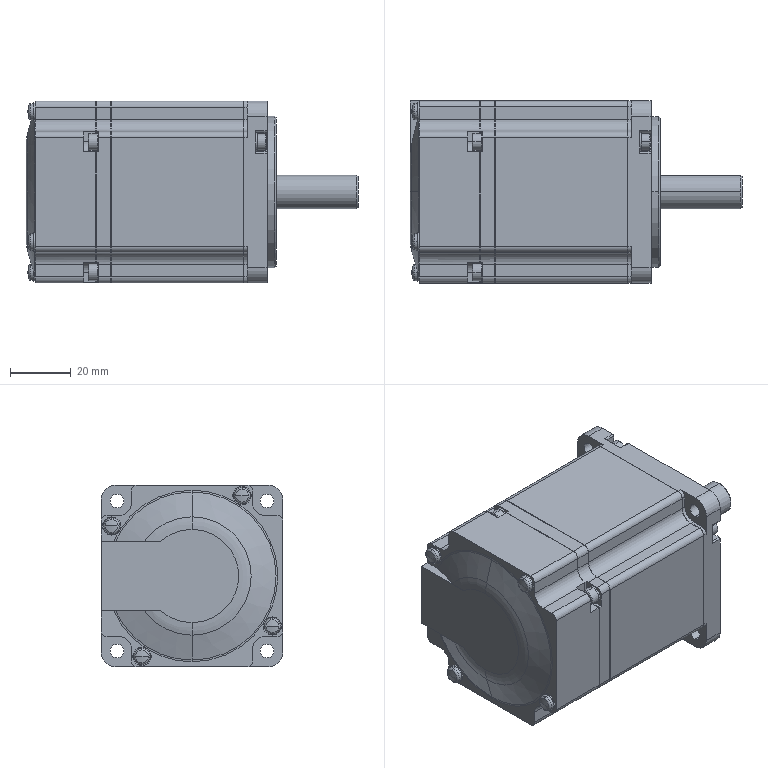Part | STEP file | MSMF022LNoStraight_b | 1 solid | 439 faces | box 109.5 x 60 x 60 mm | volume 260570 mm3 | plane 219 | cylinder 165 | cone 31 | torus 16 | sphere 8 | commonest cylinder face diameters 4 x32 6 x24 3.92 x20 5.5 x16 8 x16 6.5 x13